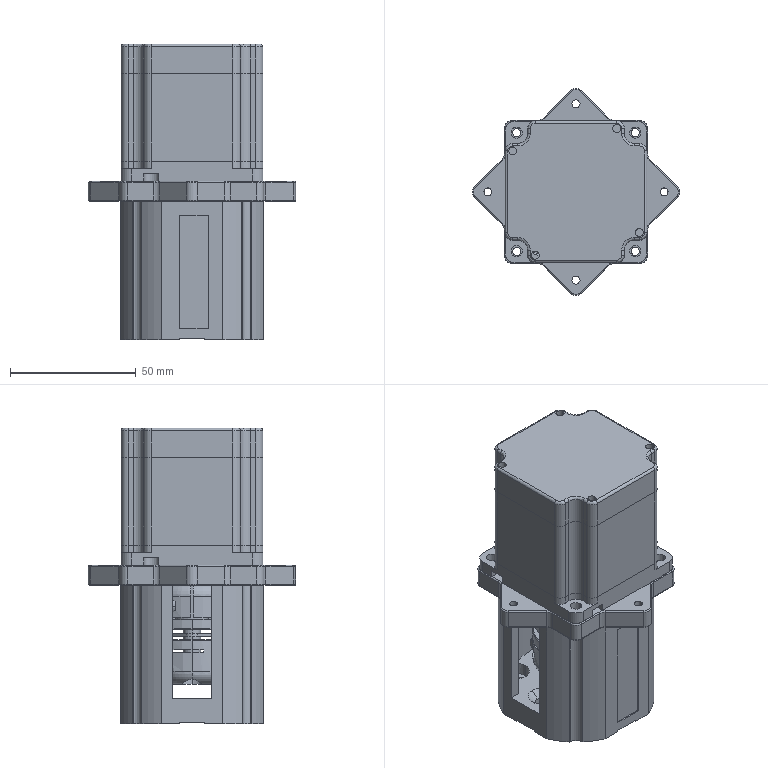Part | STEP file | Copy of 57 motor assembly (universal motor base)^K50A-1H20-S(formula driven)-L300-motor left- | 5 solids | 634 faces | box 82.368 x 82.368 x 117.5 mm | volume 245014 mm3 | cylinder 312 | plane 215 | torus 49 | cone 46 | spline 12 | commonest cylinder face diameters 6 x51 1 x40 3.2 x40 8 x39 7 x32 3.3 x21